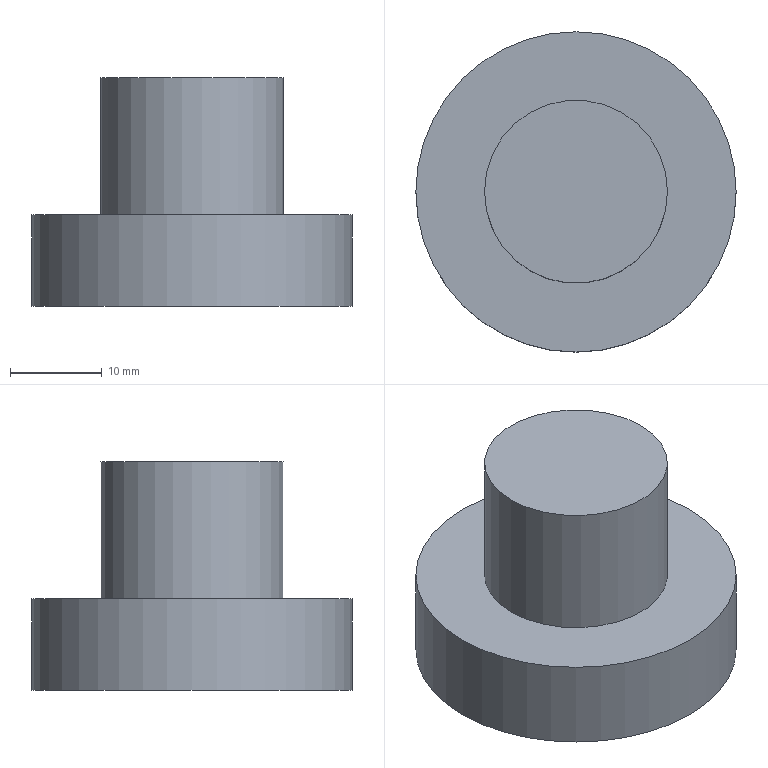Part | NX | features DATUM_CSYS 3, EXTRUDE 2, SKETCH 2 | 1 solid | 5 faces | box 35 x 35 x 25 mm | volume 14334 mm3 | plane 3 | cylinder 2 | commonest cylinder face diameters 20 x1 35 x1
STEP:
#1=CARTESIAN_POINT('',(17.5,0.,10.));
#2=VERTEX_POINT('',#1);
#3=CARTESIAN_POINT('',(0.,0.,10.));
#4=DIRECTION('',(0.,0.,-1.));
#5=DIRECTION('',(1.,0.,0.));
#6=AXIS2_PLACEMENT_3D('',#3,#4,#5);
#7=CIRCLE('',#6,17.5);
#8=EDGE_CURVE('',#2,#2,#7,.T.);
#9=ORIENTED_EDGE('',*,*,#8,.T.);
#10=EDGE_LOOP('',(#9));
#11=FACE_BOUND('',#10,.T.);
#12=CARTESIAN_POINT('',(17.5,0.,0.));
#13=VERTEX_POINT('',#12);
#14=CARTESIAN_POINT('',(0.,0.,0.));
#15=DIRECTION('',(0.,0.,-1.));
#16=DIRECTION('',(1.,0.,0.));
#17=AXIS2_PLACEMENT_3D('',#14,#15,#16);
#18=CIRCLE('',#17,17.5);
#19=EDGE_CURVE('',#13,#13,#18,.T.);
#20=ORIENTED_EDGE('',*,*,#19,.F.);
#21=EDGE_LOOP('',(#20));
#22=FACE_BOUND('',#21,.T.);
#23=CARTESIAN_POINT('',(0.,0.,10.));
#24=DIRECTION('',(0.,0.,-1.));
#25=DIRECTION('',(-1.,0.,0.));
#26=AXIS2_PLACEMENT_3D('',#23,#24,#25);
#27=CYLINDRICAL_SURFACE('',#26,17.5);
#28=ADVANCED_FACE('',(#11,#22),#27,.T.);
#29=CARTESIAN_POINT('',(10.,0.,10.));
#30=VERTEX_POINT('',#29);
#31=CARTESIAN_POINT('',(0.,0.,10.));
#32=DIRECTION('',(0.,0.,1.));
#33=DIRECTION('',(1.,0.,0.));
#34=AXIS2_PLACEMENT_3D('',#31,#32,#33);
#35=CIRCLE('',#34,10.);
#36=EDGE_CURVE('',#30,#30,#35,.T.);
#37=ORIENTED_EDGE('',*,*,#36,.F.);
#38=EDGE_LOOP('',(#37));
#39=FACE_BOUND('',#38,.T.);
#40=ORIENTED_EDGE('',*,*,#8,.F.);
#41=EDGE_LOOP('',(#40));
#42=FACE_BOUND('',#41,.T.);
#43=CARTESIAN_POINT('',(0.,0.,10.));
#44=DIRECTION('',(0.,0.,-1.));
#45=DIRECTION('',(-1.,0.,0.));
#46=AXIS2_PLACEMENT_3D('',#43,#44,#45);
#47=PLANE('',#46);
#48=ADVANCED_FACE('',(#39,#42),#47,.F.);
#49=ORIENTED_EDGE('',*,*,#19,.T.);
#50=EDGE_LOOP('',(#49));
#51=FACE_BOUND('',#50,.T.);
#52=CARTESIAN_POINT('',(0.,0.,0.));
#53=DIRECTION('',(0.,0.,-1.));
#54=DIRECTION('',(-1.,0.,0.));
#55=AXIS2_PLACEMENT_3D('',#52,#53,#54);
#56=PLANE('',#55);
#57=ADVANCED_FACE('',(#51),#56,.T.);
#58=CARTESIAN_POINT('',(10.,0.,25.));
#59=VERTEX_POINT('',#58);
#60=CARTESIAN_POINT('',(0.,0.,25.));
#61=DIRECTION('',(0.,0.,1.));
#62=DIRECTION('',(1.,0.,0.));
#63=AXIS2_PLACEMENT_3D('',#60,#61,#62);
#64=CIRCLE('',#63,10.);
#65=EDGE_CURVE('',#59,#59,#64,.T.);
#66=ORIENTED_EDGE('',*,*,#65,.F.);
#67=EDGE_LOOP('',(#66));
#68=FACE_BOUND('',#67,.T.);
#69=ORIENTED_EDGE('',*,*,#36,.T.);
#70=EDGE_LOOP('',(#69));
#71=FACE_BOUND('',#70,.T.);
#72=CARTESIAN_POINT('',(0.,0.,25.));
#73=DIRECTION('',(0.,0.,-1.));
#74=DIRECTION('',(-1.,0.,0.));
#75=AXIS2_PLACEMENT_3D('',#72,#73,#74);
#76=CYLINDRICAL_SURFACE('',#75,10.);
#77=ADVANCED_FACE('',(#68,#71),#76,.T.);
#78=ORIENTED_EDGE('',*,*,#65,.T.);
#79=EDGE_LOOP('',(#78));
#80=FACE_BOUND('',#79,.T.);
#81=CARTESIAN_POINT('',(0.,0.,25.));
#82=DIRECTION('',(0.,0.,1.));
#83=DIRECTION('',(1.,0.,0.));
#84=AXIS2_PLACEMENT_3D('',#81,#82,#83);
#85=PLANE('',#84);
#86=ADVANCED_FACE('',(#80),#85,.T.);
#87=CLOSED_SHELL('',(#28,#48,#57,#77,#86));
#88=MANIFOLD_SOLID_BREP('',#87);
#89=(LENGTH_UNIT()NAMED_UNIT(*)SI_UNIT(.MILLI.,.METRE.));
#90=UNCERTAINTY_MEASURE_WITH_UNIT(LENGTH_MEASURE(0.00001),#89,'','');
#91=(NAMED_UNIT(*)PLANE_ANGLE_UNIT()SI_UNIT($,.RADIAN.));
#92=(NAMED_UNIT(*)SI_UNIT($,.STERADIAN.)SOLID_ANGLE_UNIT());
#93=(GEOMETRIC_REPRESENTATION_CONTEXT(3)GLOBAL_UNCERTAINTY_ASSIGNED_CONTEXT((#90))GLOBAL_UNIT_ASSIGNED_CONTEXT((#89,#91,#92))REPRESENTATION_CONTEXT('',''));
#94=ADVANCED_BREP_SHAPE_REPRESENTATION('',(#88),#93);